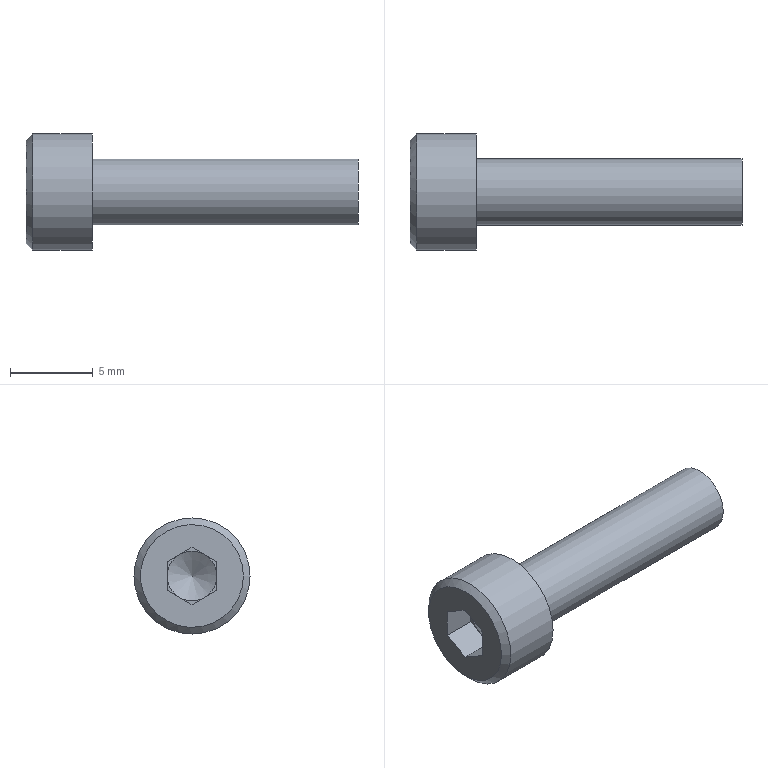Part | NX | features 5003_323_CB4-16 2 | 1 solid | 19 faces | box 20 x 7 x 7 mm | volume 335.596 mm3 | plane 15 | cylinder 2 | cone 2 | commonest cylinder face diameters 4 x1 7 x1
STEP:
#1=CARTESIAN_POINT('',(-253.475,-505.1,-109.85));
#2=VERTEX_POINT('',#1);
#3=CARTESIAN_POINT('',(-253.475,-502.,-109.85));
#4=DIRECTION('',(1.,0.,0.));
#5=DIRECTION('',(0.,-1.,0.));
#6=AXIS2_PLACEMENT_3D('',#3,#4,#5);
#7=CIRCLE('',#6,3.1);
#8=EDGE_CURVE('',#2,#2,#7,.F.);
#9=ORIENTED_EDGE('',*,*,#8,.T.);
#10=EDGE_LOOP('',(#9));
#11=FACE_BOUND('',#10,.T.);
#12=CARTESIAN_POINT('',(-253.475,-502.,-108.118));
#13=VERTEX_POINT('',#12);
#14=CARTESIAN_POINT('',(-253.475,-500.5,-108.984));
#15=VERTEX_POINT('',#14);
#16=CARTESIAN_POINT('',(-253.475,-502.,-108.118));
#17=DIRECTION('',(0.,0.866,-0.5));
#18=VECTOR('',#17,1000.);
#19=LINE('',#16,#18);
#20=EDGE_CURVE('',#13,#15,#19,.T.);
#21=ORIENTED_EDGE('',*,*,#20,.F.);
#22=CARTESIAN_POINT('',(-253.475,-503.5,-108.984));
#23=VERTEX_POINT('',#22);
#24=CARTESIAN_POINT('',(-253.475,-503.5,-108.984));
#25=DIRECTION('',(0.,0.866,0.5));
#26=VECTOR('',#25,1000.);
#27=LINE('',#24,#26);
#28=EDGE_CURVE('',#23,#13,#27,.T.);
#29=ORIENTED_EDGE('',*,*,#28,.F.);
#30=CARTESIAN_POINT('',(-253.475,-503.5,-110.716));
#31=VERTEX_POINT('',#30);
#32=CARTESIAN_POINT('',(-253.475,-503.5,-110.716));
#33=DIRECTION('',(0.,0.,1.));
#34=VECTOR('',#33,1000.);
#35=LINE('',#32,#34);
#36=EDGE_CURVE('',#31,#23,#35,.T.);
#37=ORIENTED_EDGE('',*,*,#36,.F.);
#38=CARTESIAN_POINT('',(-253.475,-502.,-111.582));
#39=VERTEX_POINT('',#38);
#40=CARTESIAN_POINT('',(-253.475,-502.,-111.582));
#41=DIRECTION('',(0.,-0.866,0.5));
#42=VECTOR('',#41,1000.);
#43=LINE('',#40,#42);
#44=EDGE_CURVE('',#39,#31,#43,.T.);
#45=ORIENTED_EDGE('',*,*,#44,.F.);
#46=CARTESIAN_POINT('',(-253.475,-500.5,-110.716));
#47=VERTEX_POINT('',#46);
#48=CARTESIAN_POINT('',(-253.475,-500.5,-110.716));
#49=DIRECTION('',(0.,-0.866,-0.5));
#50=VECTOR('',#49,1000.);
#51=LINE('',#48,#50);
#52=EDGE_CURVE('',#47,#39,#51,.T.);
#53=ORIENTED_EDGE('',*,*,#52,.F.);
#54=CARTESIAN_POINT('',(-253.475,-500.5,-108.984));
#55=DIRECTION('',(0.,0.,-1.));
#56=VECTOR('',#55,1000.);
#57=LINE('',#54,#56);
#58=EDGE_CURVE('',#15,#47,#57,.T.);
#59=ORIENTED_EDGE('',*,*,#58,.F.);
#60=EDGE_LOOP('',(#21,#29,#37,#45,#53,#59));
#61=FACE_BOUND('',#60,.T.);
#62=CARTESIAN_POINT('',(-253.475,-502.,-113.35));
#63=DIRECTION('',(1.,0.,0.));
#64=DIRECTION('',(0.,-1.,0.));
#65=AXIS2_PLACEMENT_3D('',#62,#63,#64);
#66=PLANE('',#65);
#67=ADVANCED_FACE('',(#11,#61),#66,.F.);
#68=CARTESIAN_POINT('',(-233.475,-500.,-109.85));
#69=VERTEX_POINT('',#68);
#70=CARTESIAN_POINT('',(-233.475,-502.,-109.85));
#71=DIRECTION('',(-1.,0.,0.));
#72=DIRECTION('',(0.,1.,0.));
#73=AXIS2_PLACEMENT_3D('',#70,#71,#72);
#74=CIRCLE('',#73,2.);
#75=EDGE_CURVE('',#69,#69,#74,.T.);
#76=ORIENTED_EDGE('',*,*,#75,.F.);
#77=EDGE_LOOP('',(#76));
#78=FACE_BOUND('',#77,.T.);
#79=CARTESIAN_POINT('',(-233.475,-502.,-109.85));
#80=DIRECTION('',(-1.,0.,0.));
#81=DIRECTION('',(0.,1.,0.));
#82=AXIS2_PLACEMENT_3D('',#79,#80,#81);
#83=PLANE('',#82);
#84=ADVANCED_FACE('',(#78),#83,.F.);
#85=CARTESIAN_POINT('',(-249.475,-500.,-109.85));
#86=VERTEX_POINT('',#85);
#87=CARTESIAN_POINT('',(-249.475,-502.,-109.85));
#88=DIRECTION('',(-1.,0.,0.));
#89=DIRECTION('',(0.,1.,0.));
#90=AXIS2_PLACEMENT_3D('',#87,#88,#89);
#91=CIRCLE('',#90,2.);
#92=EDGE_CURVE('',#86,#86,#91,.T.);
#93=ORIENTED_EDGE('',*,*,#92,.F.);
#94=EDGE_LOOP('',(#93));
#95=FACE_BOUND('',#94,.T.);
#96=ORIENTED_EDGE('',*,*,#75,.T.);
#97=EDGE_LOOP('',(#96));
#98=FACE_BOUND('',#97,.T.);
#99=CARTESIAN_POINT('',(-253.475,-502.,-109.85));
#100=DIRECTION('',(-1.,0.,0.));
#101=DIRECTION('',(0.,1.,0.));
#102=AXIS2_PLACEMENT_3D('',#99,#100,#101);
#103=CYLINDRICAL_SURFACE('',#102,2.);
#104=ADVANCED_FACE('',(#95,#98),#103,.T.);
#105=CARTESIAN_POINT('',(-249.475,-498.5,-109.85));
#106=VERTEX_POINT('',#105);
#107=CARTESIAN_POINT('',(-249.475,-502.,-109.85));
#108=DIRECTION('',(-1.,0.,0.));
#109=DIRECTION('',(0.,1.,0.));
#110=AXIS2_PLACEMENT_3D('',#107,#108,#109);
#111=CIRCLE('',#110,3.5);
#112=EDGE_CURVE('',#106,#106,#111,.T.);
#113=ORIENTED_EDGE('',*,*,#112,.F.);
#114=EDGE_LOOP('',(#113));
#115=FACE_BOUND('',#114,.T.);
#116=ORIENTED_EDGE('',*,*,#92,.T.);
#117=EDGE_LOOP('',(#116));
#118=FACE_BOUND('',#117,.T.);
#119=CARTESIAN_POINT('',(-249.475,-502.,-111.85));
#120=DIRECTION('',(-1.,0.,0.));
#121=DIRECTION('',(0.,1.,0.));
#122=AXIS2_PLACEMENT_3D('',#119,#120,#121);
#123=PLANE('',#122);
#124=ADVANCED_FACE('',(#115,#118),#123,.F.);
#125=CARTESIAN_POINT('',(-253.075,-505.5,-109.85));
#126=VERTEX_POINT('',#125);
#127=CARTESIAN_POINT('',(-253.075,-502.,-109.85));
#128=DIRECTION('',(1.,0.,0.));
#129=DIRECTION('',(0.,-1.,0.));
#130=AXIS2_PLACEMENT_3D('',#127,#128,#129);
#131=CIRCLE('',#130,3.5);
#132=EDGE_CURVE('',#126,#126,#131,.T.);
#133=ORIENTED_EDGE('',*,*,#132,.T.);
#134=EDGE_LOOP('',(#133));
#135=FACE_BOUND('',#134,.T.);
#136=ORIENTED_EDGE('',*,*,#112,.T.);
#137=EDGE_LOOP('',(#136));
#138=FACE_BOUND('',#137,.T.);
#139=CARTESIAN_POINT('',(-253.475,-502.,-109.85));
#140=DIRECTION('',(-1.,0.,0.));
#141=DIRECTION('',(0.,1.,0.));
#142=AXIS2_PLACEMENT_3D('',#139,#140,#141);
#143=CYLINDRICAL_SURFACE('',#142,3.5);
#144=ADVANCED_FACE('',(#135,#138),#143,.T.);
#145=ORIENTED_EDGE('',*,*,#132,.F.);
#146=EDGE_LOOP('',(#145));
#147=FACE_BOUND('',#146,.T.);
#148=ORIENTED_EDGE('',*,*,#8,.F.);
#149=EDGE_LOOP('',(#148));
#150=FACE_BOUND('',#149,.T.);
#151=CARTESIAN_POINT('',(-253.475,-502.,-109.85));
#152=DIRECTION('',(1.,0.,0.));
#153=DIRECTION('',(0.,-1.,0.));
#154=AXIS2_PLACEMENT_3D('',#151,#152,#153);
#155=CONICAL_SURFACE('',#154,3.1,0.7854);
#156=ADVANCED_FACE('',(#147,#150),#155,.T.);
#157=CARTESIAN_POINT('',(-251.475,-503.5,-108.984));
#158=VERTEX_POINT('',#157);
#159=CARTESIAN_POINT('',(-251.475,-502.75,-108.551));
#160=VERTEX_POINT('',#159);
#161=CARTESIAN_POINT('',(-251.475,-503.5,-108.984));
#162=DIRECTION('',(0.,0.866,0.5));
#163=VECTOR('',#162,1000.);
#164=LINE('',#161,#163);
#165=EDGE_CURVE('',#158,#160,#164,.T.);
#166=ORIENTED_EDGE('',*,*,#165,.F.);
#167=CARTESIAN_POINT('',(-251.475,-503.5,-108.984));
#168=DIRECTION('',(-1.,0.,0.));
#169=VECTOR('',#168,1000.);
#170=LINE('',#167,#169);
#171=EDGE_CURVE('',#158,#23,#170,.T.);
#172=ORIENTED_EDGE('',*,*,#171,.T.);
#173=ORIENTED_EDGE('',*,*,#28,.T.);
#174=CARTESIAN_POINT('',(-251.475,-502.,-108.118));
#175=VERTEX_POINT('',#174);
#176=CARTESIAN_POINT('',(-251.475,-502.,-108.118));
#177=DIRECTION('',(-1.,0.,0.));
#178=VECTOR('',#177,1000.);
#179=LINE('',#176,#178);
#180=EDGE_CURVE('',#175,#13,#179,.T.);
#181=ORIENTED_EDGE('',*,*,#180,.F.);
#182=CARTESIAN_POINT('',(-251.475,-503.5,-108.984));
#183=DIRECTION('',(0.,0.866,0.5));
#184=VECTOR('',#183,1000.);
#185=LINE('',#182,#184);
#186=EDGE_CURVE('',#160,#175,#185,.T.);
#187=ORIENTED_EDGE('',*,*,#186,.F.);
#188=EDGE_LOOP('',(#166,#172,#173,#181,#187));
#189=FACE_BOUND('',#188,.T.);
#190=CARTESIAN_POINT('',(-251.475,-503.5,-108.984));
#191=DIRECTION('',(0.,-0.5,0.866));
#192=DIRECTION('',(0.,-0.866,-0.5));
#193=AXIS2_PLACEMENT_3D('',#190,#191,#192);
#194=PLANE('',#193);
#195=ADVANCED_FACE('',(#189),#194,.F.);
#196=CARTESIAN_POINT('',(-251.475,-503.5,-110.716));
#197=VERTEX_POINT('',#196);
#198=CARTESIAN_POINT('',(-251.475,-503.5,-109.85));
#199=VERTEX_POINT('',#198);
#200=CARTESIAN_POINT('',(-251.475,-503.5,-110.716));
#201=DIRECTION('',(0.,0.,1.));
#202=VECTOR('',#201,1000.);
#203=LINE('',#200,#202);
#204=EDGE_CURVE('',#197,#199,#203,.T.);
#205=ORIENTED_EDGE('',*,*,#204,.F.);
#206=CARTESIAN_POINT('',(-251.475,-503.5,-110.716));
#207=DIRECTION('',(-1.,0.,0.));
#208=VECTOR('',#207,1000.);
#209=LINE('',#206,#208);
#210=EDGE_CURVE('',#197,#31,#209,.T.);
#211=ORIENTED_EDGE('',*,*,#210,.T.);
#212=ORIENTED_EDGE('',*,*,#36,.T.);
#213=ORIENTED_EDGE('',*,*,#171,.F.);
#214=CARTESIAN_POINT('',(-251.475,-503.5,-110.716));
#215=DIRECTION('',(0.,0.,1.));
#216=VECTOR('',#215,1000.);
#217=LINE('',#214,#216);
#218=EDGE_CURVE('',#199,#158,#217,.T.);
#219=ORIENTED_EDGE('',*,*,#218,.F.);
#220=EDGE_LOOP('',(#205,#211,#212,#213,#219));
#221=FACE_BOUND('',#220,.T.);
#222=CARTESIAN_POINT('',(-251.475,-503.5,-110.716));
#223=DIRECTION('',(0.,-1.,0.));
#224=DIRECTION('',(-1.,0.,0.));
#225=AXIS2_PLACEMENT_3D('',#222,#223,#224);
#226=PLANE('',#225);
#227=ADVANCED_FACE('',(#221),#226,.F.);
#228=CARTESIAN_POINT('',(-251.475,-502.,-111.582));
#229=VERTEX_POINT('',#228);
#230=CARTESIAN_POINT('',(-251.475,-502.75,-111.149));
#231=VERTEX_POINT('',#230);
#232=CARTESIAN_POINT('',(-251.475,-502.,-111.582));
#233=DIRECTION('',(0.,-0.866,0.5));
#234=VECTOR('',#233,1000.);
#235=LINE('',#232,#234);
#236=EDGE_CURVE('',#229,#231,#235,.T.);
#237=ORIENTED_EDGE('',*,*,#236,.F.);
#238=CARTESIAN_POINT('',(-251.475,-502.,-111.582));
#239=DIRECTION('',(-1.,0.,0.));
#240=VECTOR('',#239,1000.);
#241=LINE('',#238,#240);
#242=EDGE_CURVE('',#229,#39,#241,.T.);
#243=ORIENTED_EDGE('',*,*,#242,.T.);
#244=ORIENTED_EDGE('',*,*,#44,.T.);
#245=ORIENTED_EDGE('',*,*,#210,.F.);
#246=CARTESIAN_POINT('',(-251.475,-502.,-111.582));
#247=DIRECTION('',(0.,-0.866,0.5));
#248=VECTOR('',#247,1000.);
#249=LINE('',#246,#248);
#250=EDGE_CURVE('',#231,#197,#249,.T.);
#251=ORIENTED_EDGE('',*,*,#250,.F.);
#252=EDGE_LOOP('',(#237,#243,#244,#245,#251));
#253=FACE_BOUND('',#252,.T.);
#254=CARTESIAN_POINT('',(-251.475,-502.,-111.582));
#255=DIRECTION('',(0.,-0.5,-0.866));
#256=DIRECTION('',(0.,0.866,-0.5));
#257=AXIS2_PLACEMENT_3D('',#254,#255,#256);
#258=PLANE('',#257);
#259=ADVANCED_FACE('',(#253),#258,.F.);
#260=CARTESIAN_POINT('',(-251.475,-500.5,-110.716));
#261=VERTEX_POINT('',#260);
#262=CARTESIAN_POINT('',(-251.475,-501.25,-111.149));
#263=VERTEX_POINT('',#262);
#264=CARTESIAN_POINT('',(-251.475,-500.5,-110.716));
#265=DIRECTION('',(0.,-0.866,-0.5));
#266=VECTOR('',#265,1000.);
#267=LINE('',#264,#266);
#268=EDGE_CURVE('',#261,#263,#267,.T.);
#269=ORIENTED_EDGE('',*,*,#268,.F.);
#270=CARTESIAN_POINT('',(-251.475,-500.5,-110.716));
#271=DIRECTION('',(-1.,0.,0.));
#272=VECTOR('',#271,1000.);
#273=LINE('',#270,#272);
#274=EDGE_CURVE('',#261,#47,#273,.T.);
#275=ORIENTED_EDGE('',*,*,#274,.T.);
#276=ORIENTED_EDGE('',*,*,#52,.T.);
#277=ORIENTED_EDGE('',*,*,#242,.F.);
#278=CARTESIAN_POINT('',(-251.475,-500.5,-110.716));
#279=DIRECTION('',(0.,-0.866,-0.5));
#280=VECTOR('',#279,1000.);
#281=LINE('',#278,#280);
#282=EDGE_CURVE('',#263,#229,#281,.T.);
#283=ORIENTED_EDGE('',*,*,#282,.F.);
#284=EDGE_LOOP('',(#269,#275,#276,#277,#283));
#285=FACE_BOUND('',#284,.T.);
#286=CARTESIAN_POINT('',(-251.475,-500.5,-110.716));
#287=DIRECTION('',(0.,0.5,-0.866));
#288=DIRECTION('',(0.,0.866,0.5));
#289=AXIS2_PLACEMENT_3D('',#286,#287,#288);
#290=PLANE('',#289);
#291=ADVANCED_FACE('',(#285),#290,.F.);
#292=CARTESIAN_POINT('',(-251.475,-500.5,-108.984));
#293=VERTEX_POINT('',#292);
#294=CARTESIAN_POINT('',(-251.475,-500.5,-109.85));
#295=VERTEX_POINT('',#294);
#296=CARTESIAN_POINT('',(-251.475,-500.5,-108.984));
#297=DIRECTION('',(0.,0.,-1.));
#298=VECTOR('',#297,1000.);
#299=LINE('',#296,#298);
#300=EDGE_CURVE('',#293,#295,#299,.T.);
#301=ORIENTED_EDGE('',*,*,#300,.F.);
#302=CARTESIAN_POINT('',(-251.475,-500.5,-108.984));
#303=DIRECTION('',(-1.,0.,0.));
#304=VECTOR('',#303,1000.);
#305=LINE('',#302,#304);
#306=EDGE_CURVE('',#293,#15,#305,.T.);
#307=ORIENTED_EDGE('',*,*,#306,.T.);
#308=ORIENTED_EDGE('',*,*,#58,.T.);
#309=ORIENTED_EDGE('',*,*,#274,.F.);
#310=CARTESIAN_POINT('',(-251.475,-500.5,-108.984));
#311=DIRECTION('',(0.,0.,-1.));
#312=VECTOR('',#311,1000.);
#313=LINE('',#310,#312);
#314=EDGE_CURVE('',#295,#261,#313,.T.);
#315=ORIENTED_EDGE('',*,*,#314,.F.);
#316=EDGE_LOOP('',(#301,#307,#308,#309,#315));
#317=FACE_BOUND('',#316,.T.);
#318=CARTESIAN_POINT('',(-251.475,-500.5,-108.984));
#319=DIRECTION('',(0.,1.,0.));
#320=DIRECTION('',(1.,0.,0.));
#321=AXIS2_PLACEMENT_3D('',#318,#319,#320);
#322=PLANE('',#321);
#323=ADVANCED_FACE('',(#317),#322,.F.);
#324=CARTESIAN_POINT('',(-251.475,-501.25,-108.551));
#325=VERTEX_POINT('',#324);
#326=CARTESIAN_POINT('',(-251.475,-502.,-108.118));
#327=DIRECTION('',(0.,0.866,-0.5));
#328=VECTOR('',#327,1000.);
#329=LINE('',#326,#328);
#330=EDGE_CURVE('',#175,#325,#329,.T.);
#331=ORIENTED_EDGE('',*,*,#330,.F.);
#332=ORIENTED_EDGE('',*,*,#180,.T.);
#333=ORIENTED_EDGE('',*,*,#20,.T.);
#334=ORIENTED_EDGE('',*,*,#306,.F.);
#335=CARTESIAN_POINT('',(-251.475,-502.,-108.118));
#336=DIRECTION('',(0.,0.866,-0.5));
#337=VECTOR('',#336,1000.);
#338=LINE('',#335,#337);
#339=EDGE_CURVE('',#325,#293,#338,.T.);
#340=ORIENTED_EDGE('',*,*,#339,.F.);
#341=EDGE_LOOP('',(#331,#332,#333,#334,#340));
#342=FACE_BOUND('',#341,.T.);
#343=CARTESIAN_POINT('',(-251.475,-502.,-108.118));
#344=DIRECTION('',(0.,0.5,0.866));
#345=DIRECTION('',(0.,-0.866,0.5));
#346=AXIS2_PLACEMENT_3D('',#343,#344,#345);
#347=PLANE('',#346);
#348=ADVANCED_FACE('',(#342),#347,.F.);
#349=ORIENTED_EDGE('',*,*,#314,.T.);
#350=ORIENTED_EDGE('',*,*,#268,.T.);
#351=CARTESIAN_POINT('',(-251.475,-502.,-109.85));
#352=DIRECTION('',(-1.,0.,0.));
#353=DIRECTION('',(0.,0.,1.));
#354=AXIS2_PLACEMENT_3D('',#351,#352,#353);
#355=CIRCLE('',#354,1.5);
#356=EDGE_CURVE('',#295,#263,#355,.T.);
#357=ORIENTED_EDGE('',*,*,#356,.F.);
#358=EDGE_LOOP('',(#349,#350,#357));
#359=FACE_BOUND('',#358,.T.);
#360=CARTESIAN_POINT('',(-251.475,-502.,-109.85));
#361=DIRECTION('',(-1.,0.,0.));
#362=DIRECTION('',(0.,1.,0.));
#363=AXIS2_PLACEMENT_3D('',#360,#361,#362);
#364=PLANE('',#363);
#365=ADVANCED_FACE('',(#359),#364,.T.);
#366=ORIENTED_EDGE('',*,*,#282,.T.);
#367=ORIENTED_EDGE('',*,*,#236,.T.);
#368=CARTESIAN_POINT('',(-251.475,-502.,-109.85));
#369=DIRECTION('',(-1.,0.,0.));
#370=DIRECTION('',(0.,0.,1.));
#371=AXIS2_PLACEMENT_3D('',#368,#369,#370);
#372=CIRCLE('',#371,1.5);
#373=EDGE_CURVE('',#263,#231,#372,.T.);
#374=ORIENTED_EDGE('',*,*,#373,.F.);
#375=EDGE_LOOP('',(#366,#367,#374));
#376=FACE_BOUND('',#375,.T.);
#377=CARTESIAN_POINT('',(-251.475,-502.,-109.85));
#378=DIRECTION('',(-1.,0.,0.));
#379=DIRECTION('',(0.,1.,0.));
#380=AXIS2_PLACEMENT_3D('',#377,#378,#379);
#381=PLANE('',#380);
#382=ADVANCED_FACE('',(#376),#381,.T.);
#383=ORIENTED_EDGE('',*,*,#250,.T.);
#384=ORIENTED_EDGE('',*,*,#204,.T.);
#385=CARTESIAN_POINT('',(-251.475,-502.,-109.85));
#386=DIRECTION('',(-1.,0.,0.));
#387=DIRECTION('',(0.,0.,1.));
#388=AXIS2_PLACEMENT_3D('',#385,#386,#387);
#389=CIRCLE('',#388,1.5);
#390=EDGE_CURVE('',#231,#199,#389,.T.);
#391=ORIENTED_EDGE('',*,*,#390,.F.);
#392=EDGE_LOOP('',(#383,#384,#391));
#393=FACE_BOUND('',#392,.T.);
#394=CARTESIAN_POINT('',(-251.475,-502.,-109.85));
#395=DIRECTION('',(-1.,0.,0.));
#396=DIRECTION('',(0.,1.,0.));
#397=AXIS2_PLACEMENT_3D('',#394,#395,#396);
#398=PLANE('',#397);
#399=ADVANCED_FACE('',(#393),#398,.T.);
#400=ORIENTED_EDGE('',*,*,#218,.T.);
#401=ORIENTED_EDGE('',*,*,#165,.T.);
#402=CARTESIAN_POINT('',(-251.475,-502.,-109.85));
#403=DIRECTION('',(-1.,0.,0.));
#404=DIRECTION('',(0.,0.,1.));
#405=AXIS2_PLACEMENT_3D('',#402,#403,#404);
#406=CIRCLE('',#405,1.5);
#407=EDGE_CURVE('',#199,#160,#406,.T.);
#408=ORIENTED_EDGE('',*,*,#407,.F.);
#409=EDGE_LOOP('',(#400,#401,#408));
#410=FACE_BOUND('',#409,.T.);
#411=CARTESIAN_POINT('',(-251.475,-502.,-109.85));
#412=DIRECTION('',(-1.,0.,0.));
#413=DIRECTION('',(0.,1.,0.));
#414=AXIS2_PLACEMENT_3D('',#411,#412,#413);
#415=PLANE('',#414);
#416=ADVANCED_FACE('',(#410),#415,.T.);
#417=ORIENTED_EDGE('',*,*,#186,.T.);
#418=ORIENTED_EDGE('',*,*,#330,.T.);
#419=CARTESIAN_POINT('',(-251.475,-502.,-109.85));
#420=DIRECTION('',(-1.,0.,0.));
#421=DIRECTION('',(0.,0.,1.));
#422=AXIS2_PLACEMENT_3D('',#419,#420,#421);
#423=CIRCLE('',#422,1.5);
#424=EDGE_CURVE('',#160,#325,#423,.T.);
#425=ORIENTED_EDGE('',*,*,#424,.F.);
#426=EDGE_LOOP('',(#417,#418,#425));
#427=FACE_BOUND('',#426,.T.);
#428=CARTESIAN_POINT('',(-251.475,-502.,-109.85));
#429=DIRECTION('',(-1.,0.,0.));
#430=DIRECTION('',(0.,1.,0.));
#431=AXIS2_PLACEMENT_3D('',#428,#429,#430);
#432=PLANE('',#431);
#433=ADVANCED_FACE('',(#427),#432,.T.);
#434=ORIENTED_EDGE('',*,*,#339,.T.);
#435=ORIENTED_EDGE('',*,*,#300,.T.);
#436=CARTESIAN_POINT('',(-251.475,-502.,-109.85));
#437=DIRECTION('',(-1.,0.,0.));
#438=DIRECTION('',(0.,0.,1.));
#439=AXIS2_PLACEMENT_3D('',#436,#437,#438);
#440=CIRCLE('',#439,1.5);
#441=EDGE_CURVE('',#325,#295,#440,.T.);
#442=ORIENTED_EDGE('',*,*,#441,.F.);
#443=EDGE_LOOP('',(#434,#435,#442));
#444=FACE_BOUND('',#443,.T.);
#445=CARTESIAN_POINT('',(-251.475,-502.,-109.85));
#446=DIRECTION('',(-1.,0.,0.));
#447=DIRECTION('',(0.,1.,0.));
#448=AXIS2_PLACEMENT_3D('',#445,#446,#447);
#449=PLANE('',#448);
#450=ADVANCED_FACE('',(#444),#449,.T.);
#451=ORIENTED_EDGE('',*,*,#441,.T.);
#452=ORIENTED_EDGE('',*,*,#356,.T.);
#453=ORIENTED_EDGE('',*,*,#373,.T.);
#454=ORIENTED_EDGE('',*,*,#390,.T.);
#455=ORIENTED_EDGE('',*,*,#407,.T.);
#456=ORIENTED_EDGE('',*,*,#424,.T.);
#457=EDGE_LOOP('',(#451,#452,#453,#454,#455,#456));
#458=FACE_BOUND('',#457,.T.);
#459=CARTESIAN_POINT('',(-250.574,-502.,-109.85));
#460=VERTEX_POINT('',#459);
#461=VERTEX_LOOP('',#460);
#462=FACE_BOUND('',#461,.T.);
#463=CARTESIAN_POINT('',(-250.574,-502.,-109.85));
#464=DIRECTION('',(-1.,0.,0.));
#465=DIRECTION('',(0.,0.,1.));
#466=AXIS2_PLACEMENT_3D('',#463,#464,#465);
#467=CONICAL_SURFACE('',#466,0.,1.03);
#468=ADVANCED_FACE('',(#458,#462),#467,.F.);
#469=CLOSED_SHELL('',(#67,#84,#104,#124,#144,#156,#195,#227,#259,#291,#323,#348,#365,#382,#399,#416,#433,#450,#468));
#470=MANIFOLD_SOLID_BREP('',#469);
#471=(LENGTH_UNIT()NAMED_UNIT(*)SI_UNIT(.MILLI.,.METRE.));
#472=UNCERTAINTY_MEASURE_WITH_UNIT(LENGTH_MEASURE(0.00001),#471,'','');
#473=(NAMED_UNIT(*)PLANE_ANGLE_UNIT()SI_UNIT($,.RADIAN.));
#474=(NAMED_UNIT(*)SI_UNIT($,.STERADIAN.)SOLID_ANGLE_UNIT());
#475=(GEOMETRIC_REPRESENTATION_CONTEXT(3)GLOBAL_UNCERTAINTY_ASSIGNED_CONTEXT((#472))GLOBAL_UNIT_ASSIGNED_CONTEXT((#471,#473,#474))REPRESENTATION_CONTEXT('',''));
#476=ADVANCED_BREP_SHAPE_REPRESENTATION('',(#470),#475);